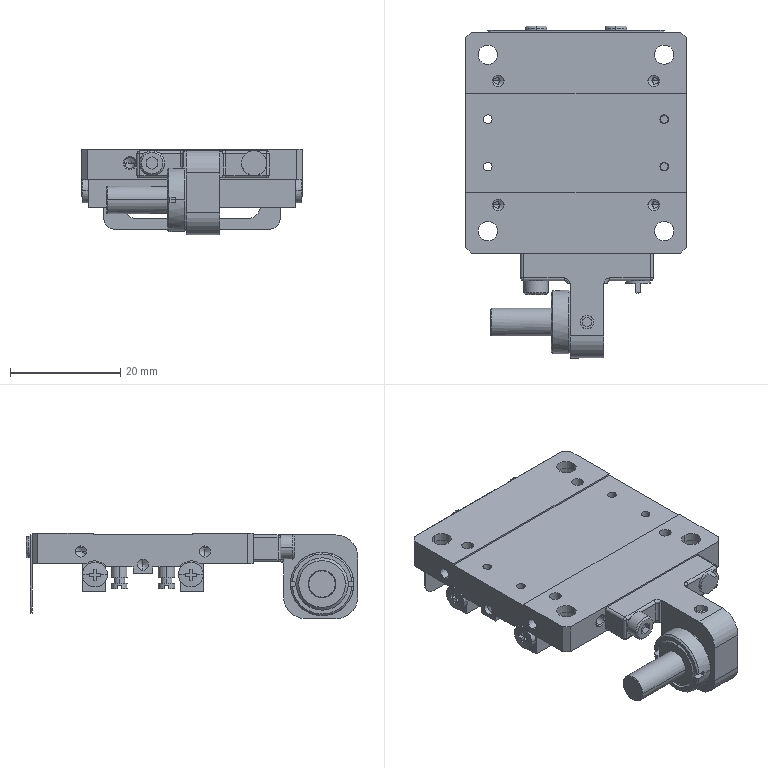Part | SolidWorks | features BaseBody 14 | 14 solids | 633 faces | box 40 x 60.2 x 15.5 mm | volume 12589 mm3 | plane 235 | cylinder 225 | cone 131 | spline 22 | torus 20 | commonest cylinder face diameters 2.1 x48 2.013 x24 2 x22 1.567 x16 3 x16 1 x13